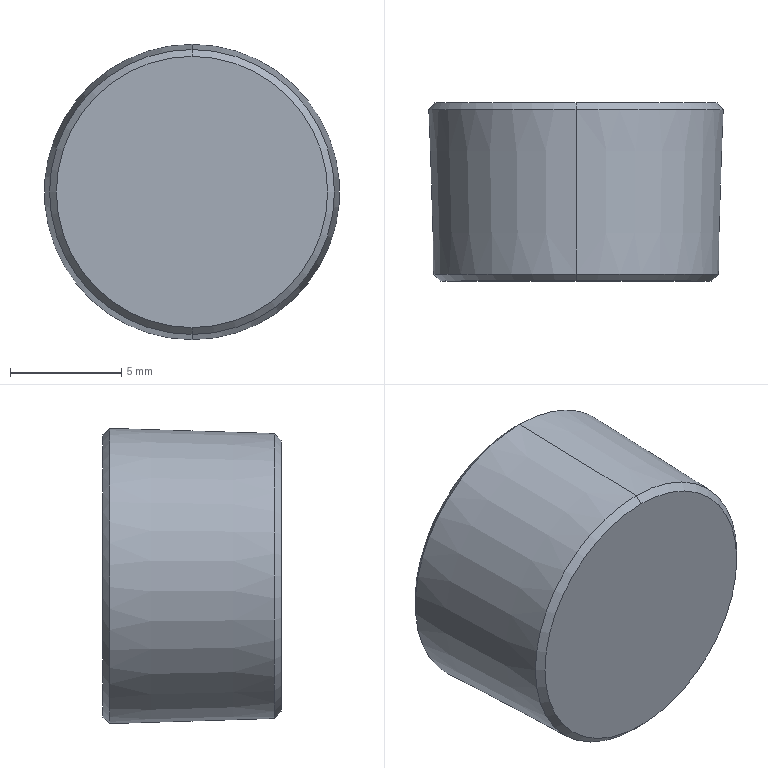Part | STEP file | 1 solid | 17 faces | box 13.263 x 8 x 13.263 mm | volume 903.778 mm3 | plane 9 | cone 8